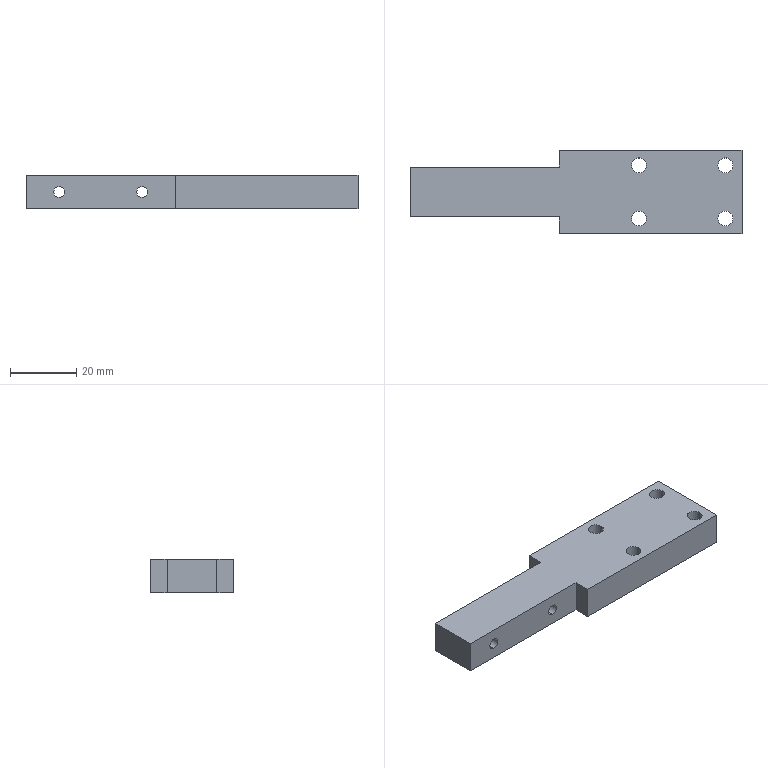Part | SolidWorks | features HoleWzd 2, Cut 1, Extrusion 1 | 1 solid | 34 faces | box 100 x 25 x 10 mm | volume 18975 mm3 | cylinder 20 | plane 14 | commonest cylinder face diameters 4.5 x8 8 x8 3.3 x4
STEP:
#1=CARTESIAN_POINT('',(-15.,-7.5,3.35));
#2=VERTEX_POINT('',#1);
#3=CARTESIAN_POINT('',(-15.,-7.5,6.65));
#4=VERTEX_POINT('',#3);
#5=CARTESIAN_POINT('',(-15.,-7.5,5.));
#6=DIRECTION('',(0.,1.,0.));
#7=DIRECTION('',(-1.,0.,0.));
#8=AXIS2_PLACEMENT_3D('',#5,#6,#7);
#9=CIRCLE('',#8,1.65);
#10=EDGE_CURVE('',#2,#4,#9,.T.);
#11=ORIENTED_EDGE('',*,*,#10,.F.);
#12=CARTESIAN_POINT('',(-15.,7.5,3.35));
#13=VERTEX_POINT('',#12);
#14=CARTESIAN_POINT('',(-15.,7.5,3.35));
#15=DIRECTION('',(0.,1.,0.));
#16=VECTOR('',#15,1000.);
#17=LINE('',#14,#16);
#18=EDGE_CURVE('',#2,#13,#17,.T.);
#19=ORIENTED_EDGE('',*,*,#18,.T.);
#20=CARTESIAN_POINT('',(-15.,7.5,6.65));
#21=VERTEX_POINT('',#20);
#22=CARTESIAN_POINT('',(-15.,7.5,5.));
#23=DIRECTION('',(0.,1.,0.));
#24=DIRECTION('',(0.,0.,1.));
#25=AXIS2_PLACEMENT_3D('',#22,#23,#24);
#26=CIRCLE('',#25,1.65);
#27=EDGE_CURVE('',#13,#21,#26,.T.);
#28=ORIENTED_EDGE('',*,*,#27,.T.);
#29=CARTESIAN_POINT('',(-15.,7.5,6.65));
#30=DIRECTION('',(0.,1.,0.));
#31=VECTOR('',#30,1000.);
#32=LINE('',#29,#31);
#33=EDGE_CURVE('',#4,#21,#32,.T.);
#34=ORIENTED_EDGE('',*,*,#33,.F.);
#35=EDGE_LOOP('',(#11,#19,#28,#34));
#36=FACE_OUTER_BOUND('',#35,.T.);
#37=CARTESIAN_POINT('',(-15.,7.5,5.));
#38=DIRECTION('',(0.,1.,0.));
#39=DIRECTION('',(0.,0.,1.));
#40=AXIS2_PLACEMENT_3D('',#37,#38,#39);
#41=CYLINDRICAL_SURFACE('',#40,1.65);
#42=ADVANCED_FACE('',(#36),#41,.F.);
#43=CARTESIAN_POINT('',(-40.,-7.5,3.35));
#44=VERTEX_POINT('',#43);
#45=CARTESIAN_POINT('',(-40.,-7.5,6.65));
#46=VERTEX_POINT('',#45);
#47=CARTESIAN_POINT('',(-40.,-7.5,5.));
#48=DIRECTION('',(0.,1.,0.));
#49=DIRECTION('',(-1.,0.,0.));
#50=AXIS2_PLACEMENT_3D('',#47,#48,#49);
#51=CIRCLE('',#50,1.65);
#52=EDGE_CURVE('',#44,#46,#51,.T.);
#53=ORIENTED_EDGE('',*,*,#52,.F.);
#54=CARTESIAN_POINT('',(-40.,7.5,3.35));
#55=VERTEX_POINT('',#54);
#56=CARTESIAN_POINT('',(-40.,7.5,3.35));
#57=DIRECTION('',(0.,1.,0.));
#58=VECTOR('',#57,1000.);
#59=LINE('',#56,#58);
#60=EDGE_CURVE('',#44,#55,#59,.T.);
#61=ORIENTED_EDGE('',*,*,#60,.T.);
#62=CARTESIAN_POINT('',(-40.,7.5,6.65));
#63=VERTEX_POINT('',#62);
#64=CARTESIAN_POINT('',(-40.,7.5,5.));
#65=DIRECTION('',(0.,1.,0.));
#66=DIRECTION('',(0.,0.,1.));
#67=AXIS2_PLACEMENT_3D('',#64,#65,#66);
#68=CIRCLE('',#67,1.65);
#69=EDGE_CURVE('',#55,#63,#68,.T.);
#70=ORIENTED_EDGE('',*,*,#69,.T.);
#71=CARTESIAN_POINT('',(-40.,7.5,6.65));
#72=DIRECTION('',(0.,1.,0.));
#73=VECTOR('',#72,1000.);
#74=LINE('',#71,#73);
#75=EDGE_CURVE('',#46,#63,#74,.T.);
#76=ORIENTED_EDGE('',*,*,#75,.F.);
#77=EDGE_LOOP('',(#53,#61,#70,#76));
#78=FACE_OUTER_BOUND('',#77,.T.);
#79=CARTESIAN_POINT('',(-40.,7.5,5.));
#80=DIRECTION('',(0.,1.,0.));
#81=DIRECTION('',(0.,0.,1.));
#82=AXIS2_PLACEMENT_3D('',#79,#80,#81);
#83=CYLINDRICAL_SURFACE('',#82,1.65);
#84=ADVANCED_FACE('',(#78),#83,.F.);
#85=CARTESIAN_POINT('',(23.,-8.,4.6));
#86=VERTEX_POINT('',#85);
#87=CARTESIAN_POINT('',(15.,-8.,4.6));
#88=VERTEX_POINT('',#87);
#89=CARTESIAN_POINT('',(19.,-8.,4.6));
#90=DIRECTION('',(0.,0.,-1.));
#91=DIRECTION('',(-1.,0.,0.));
#92=AXIS2_PLACEMENT_3D('',#89,#90,#91);
#93=CIRCLE('',#92,4.);
#94=EDGE_CURVE('',#86,#88,#93,.T.);
#95=ORIENTED_EDGE('',*,*,#94,.F.);
#96=CARTESIAN_POINT('',(23.,-8.,0.));
#97=VERTEX_POINT('',#96);
#98=CARTESIAN_POINT('',(23.,-8.,0.));
#99=DIRECTION('',(0.,0.,-1.));
#100=VECTOR('',#99,1000.);
#101=LINE('',#98,#100);
#102=EDGE_CURVE('',#86,#97,#101,.T.);
#103=ORIENTED_EDGE('',*,*,#102,.T.);
#104=CARTESIAN_POINT('',(15.,-8.,0.));
#105=VERTEX_POINT('',#104);
#106=CARTESIAN_POINT('',(19.,-8.,0.));
#107=DIRECTION('',(0.,0.,-1.));
#108=DIRECTION('',(-1.,0.,0.));
#109=AXIS2_PLACEMENT_3D('',#106,#107,#108);
#110=CIRCLE('',#109,4.);
#111=EDGE_CURVE('',#97,#105,#110,.T.);
#112=ORIENTED_EDGE('',*,*,#111,.T.);
#113=CARTESIAN_POINT('',(15.,-8.,0.));
#114=DIRECTION('',(0.,0.,-1.));
#115=VECTOR('',#114,1000.);
#116=LINE('',#113,#115);
#117=EDGE_CURVE('',#88,#105,#116,.T.);
#118=ORIENTED_EDGE('',*,*,#117,.F.);
#119=EDGE_LOOP('',(#95,#103,#112,#118));
#120=FACE_OUTER_BOUND('',#119,.T.);
#121=CARTESIAN_POINT('',(19.,-8.,0.));
#122=DIRECTION('',(0.,0.,-1.));
#123=DIRECTION('',(-1.,0.,0.));
#124=AXIS2_PLACEMENT_3D('',#121,#122,#123);
#125=CYLINDRICAL_SURFACE('',#124,4.);
#126=ADVANCED_FACE('',(#120),#125,.F.);
#127=CARTESIAN_POINT('',(21.25,-8.,10.));
#128=VERTEX_POINT('',#127);
#129=CARTESIAN_POINT('',(16.75,-8.,10.));
#130=VERTEX_POINT('',#129);
#131=CARTESIAN_POINT('',(19.,-8.,10.));
#132=DIRECTION('',(0.,0.,-1.));
#133=DIRECTION('',(-1.,0.,0.));
#134=AXIS2_PLACEMENT_3D('',#131,#132,#133);
#135=CIRCLE('',#134,2.25);
#136=EDGE_CURVE('',#128,#130,#135,.T.);
#137=ORIENTED_EDGE('',*,*,#136,.F.);
#138=CARTESIAN_POINT('',(21.25,-8.,4.6));
#139=VERTEX_POINT('',#138);
#140=CARTESIAN_POINT('',(21.25,-8.,0.));
#141=DIRECTION('',(0.,0.,-1.));
#142=VECTOR('',#141,1000.);
#143=LINE('',#140,#142);
#144=EDGE_CURVE('',#128,#139,#143,.T.);
#145=ORIENTED_EDGE('',*,*,#144,.T.);
#146=CARTESIAN_POINT('',(16.75,-8.,4.6));
#147=VERTEX_POINT('',#146);
#148=CARTESIAN_POINT('',(19.,-8.,4.6));
#149=DIRECTION('',(0.,0.,-1.));
#150=DIRECTION('',(-1.,0.,0.));
#151=AXIS2_PLACEMENT_3D('',#148,#149,#150);
#152=CIRCLE('',#151,2.25);
#153=EDGE_CURVE('',#139,#147,#152,.T.);
#154=ORIENTED_EDGE('',*,*,#153,.T.);
#155=CARTESIAN_POINT('',(16.75,-8.,0.));
#156=DIRECTION('',(0.,0.,-1.));
#157=VECTOR('',#156,1000.);
#158=LINE('',#155,#157);
#159=EDGE_CURVE('',#130,#147,#158,.T.);
#160=ORIENTED_EDGE('',*,*,#159,.F.);
#161=EDGE_LOOP('',(#137,#145,#154,#160));
#162=FACE_OUTER_BOUND('',#161,.T.);
#163=CARTESIAN_POINT('',(19.,-8.,0.));
#164=DIRECTION('',(0.,0.,-1.));
#165=DIRECTION('',(-1.,0.,0.));
#166=AXIS2_PLACEMENT_3D('',#163,#164,#165);
#167=CYLINDRICAL_SURFACE('',#166,2.25);
#168=ADVANCED_FACE('',(#162),#167,.F.);
#169=CARTESIAN_POINT('',(23.,8.,4.6));
#170=VERTEX_POINT('',#169);
#171=CARTESIAN_POINT('',(15.,8.,4.6));
#172=VERTEX_POINT('',#171);
#173=CARTESIAN_POINT('',(19.,8.,4.6));
#174=DIRECTION('',(0.,0.,-1.));
#175=DIRECTION('',(-1.,0.,0.));
#176=AXIS2_PLACEMENT_3D('',#173,#174,#175);
#177=CIRCLE('',#176,4.);
#178=EDGE_CURVE('',#170,#172,#177,.T.);
#179=ORIENTED_EDGE('',*,*,#178,.F.);
#180=CARTESIAN_POINT('',(23.,8.,0.));
#181=VERTEX_POINT('',#180);
#182=CARTESIAN_POINT('',(23.,8.,0.));
#183=DIRECTION('',(0.,0.,-1.));
#184=VECTOR('',#183,1000.);
#185=LINE('',#182,#184);
#186=EDGE_CURVE('',#170,#181,#185,.T.);
#187=ORIENTED_EDGE('',*,*,#186,.T.);
#188=CARTESIAN_POINT('',(15.,8.,0.));
#189=VERTEX_POINT('',#188);
#190=CARTESIAN_POINT('',(19.,8.,0.));
#191=DIRECTION('',(0.,0.,-1.));
#192=DIRECTION('',(-1.,0.,0.));
#193=AXIS2_PLACEMENT_3D('',#190,#191,#192);
#194=CIRCLE('',#193,4.);
#195=EDGE_CURVE('',#181,#189,#194,.T.);
#196=ORIENTED_EDGE('',*,*,#195,.T.);
#197=CARTESIAN_POINT('',(15.,8.,0.));
#198=DIRECTION('',(0.,0.,-1.));
#199=VECTOR('',#198,1000.);
#200=LINE('',#197,#199);
#201=EDGE_CURVE('',#172,#189,#200,.T.);
#202=ORIENTED_EDGE('',*,*,#201,.F.);
#203=EDGE_LOOP('',(#179,#187,#196,#202));
#204=FACE_OUTER_BOUND('',#203,.T.);
#205=CARTESIAN_POINT('',(19.,8.,0.));
#206=DIRECTION('',(0.,0.,-1.));
#207=DIRECTION('',(-1.,0.,0.));
#208=AXIS2_PLACEMENT_3D('',#205,#206,#207);
#209=CYLINDRICAL_SURFACE('',#208,4.);
#210=ADVANCED_FACE('',(#204),#209,.F.);
#211=CARTESIAN_POINT('',(21.25,8.,10.));
#212=VERTEX_POINT('',#211);
#213=CARTESIAN_POINT('',(16.75,8.,10.));
#214=VERTEX_POINT('',#213);
#215=CARTESIAN_POINT('',(19.,8.,10.));
#216=DIRECTION('',(0.,0.,-1.));
#217=DIRECTION('',(-1.,0.,0.));
#218=AXIS2_PLACEMENT_3D('',#215,#216,#217);
#219=CIRCLE('',#218,2.25);
#220=EDGE_CURVE('',#212,#214,#219,.T.);
#221=ORIENTED_EDGE('',*,*,#220,.F.);
#222=CARTESIAN_POINT('',(21.25,8.,4.6));
#223=VERTEX_POINT('',#222);
#224=CARTESIAN_POINT('',(21.25,8.,0.));
#225=DIRECTION('',(0.,0.,-1.));
#226=VECTOR('',#225,1000.);
#227=LINE('',#224,#226);
#228=EDGE_CURVE('',#212,#223,#227,.T.);
#229=ORIENTED_EDGE('',*,*,#228,.T.);
#230=CARTESIAN_POINT('',(16.75,8.,4.6));
#231=VERTEX_POINT('',#230);
#232=CARTESIAN_POINT('',(19.,8.,4.6));
#233=DIRECTION('',(0.,0.,-1.));
#234=DIRECTION('',(-1.,0.,0.));
#235=AXIS2_PLACEMENT_3D('',#232,#233,#234);
#236=CIRCLE('',#235,2.25);
#237=EDGE_CURVE('',#223,#231,#236,.T.);
#238=ORIENTED_EDGE('',*,*,#237,.T.);
#239=CARTESIAN_POINT('',(16.75,8.,0.));
#240=DIRECTION('',(0.,0.,-1.));
#241=VECTOR('',#240,1000.);
#242=LINE('',#239,#241);
#243=EDGE_CURVE('',#214,#231,#242,.T.);
#244=ORIENTED_EDGE('',*,*,#243,.F.);
#245=EDGE_LOOP('',(#221,#229,#238,#244));
#246=FACE_OUTER_BOUND('',#245,.T.);
#247=CARTESIAN_POINT('',(19.,8.,0.));
#248=DIRECTION('',(0.,0.,-1.));
#249=DIRECTION('',(-1.,0.,0.));
#250=AXIS2_PLACEMENT_3D('',#247,#248,#249);
#251=CYLINDRICAL_SURFACE('',#250,2.25);
#252=ADVANCED_FACE('',(#246),#251,.F.);
#253=CARTESIAN_POINT('',(49.,8.,4.6));
#254=VERTEX_POINT('',#253);
#255=CARTESIAN_POINT('',(41.,8.,4.6));
#256=VERTEX_POINT('',#255);
#257=CARTESIAN_POINT('',(45.,8.,4.6));
#258=DIRECTION('',(0.,0.,-1.));
#259=DIRECTION('',(-1.,0.,0.));
#260=AXIS2_PLACEMENT_3D('',#257,#258,#259);
#261=CIRCLE('',#260,4.);
#262=EDGE_CURVE('',#254,#256,#261,.T.);
#263=ORIENTED_EDGE('',*,*,#262,.F.);
#264=CARTESIAN_POINT('',(49.,8.,0.));
#265=VERTEX_POINT('',#264);
#266=CARTESIAN_POINT('',(49.,8.,0.));
#267=DIRECTION('',(0.,0.,-1.));
#268=VECTOR('',#267,1000.);
#269=LINE('',#266,#268);
#270=EDGE_CURVE('',#254,#265,#269,.T.);
#271=ORIENTED_EDGE('',*,*,#270,.T.);
#272=CARTESIAN_POINT('',(41.,8.,0.));
#273=VERTEX_POINT('',#272);
#274=CARTESIAN_POINT('',(45.,8.,0.));
#275=DIRECTION('',(0.,0.,-1.));
#276=DIRECTION('',(-1.,0.,0.));
#277=AXIS2_PLACEMENT_3D('',#274,#275,#276);
#278=CIRCLE('',#277,4.);
#279=EDGE_CURVE('',#265,#273,#278,.T.);
#280=ORIENTED_EDGE('',*,*,#279,.T.);
#281=CARTESIAN_POINT('',(41.,8.,0.));
#282=DIRECTION('',(0.,0.,-1.));
#283=VECTOR('',#282,1000.);
#284=LINE('',#281,#283);
#285=EDGE_CURVE('',#256,#273,#284,.T.);
#286=ORIENTED_EDGE('',*,*,#285,.F.);
#287=EDGE_LOOP('',(#263,#271,#280,#286));
#288=FACE_OUTER_BOUND('',#287,.T.);
#289=CARTESIAN_POINT('',(45.,8.,0.));
#290=DIRECTION('',(0.,0.,-1.));
#291=DIRECTION('',(-1.,0.,0.));
#292=AXIS2_PLACEMENT_3D('',#289,#290,#291);
#293=CYLINDRICAL_SURFACE('',#292,4.);
#294=ADVANCED_FACE('',(#288),#293,.F.);
#295=CARTESIAN_POINT('',(47.25,8.,10.));
#296=VERTEX_POINT('',#295);
#297=CARTESIAN_POINT('',(42.75,8.,10.));
#298=VERTEX_POINT('',#297);
#299=CARTESIAN_POINT('',(45.,8.,10.));
#300=DIRECTION('',(0.,0.,-1.));
#301=DIRECTION('',(-1.,0.,0.));
#302=AXIS2_PLACEMENT_3D('',#299,#300,#301);
#303=CIRCLE('',#302,2.25);
#304=EDGE_CURVE('',#296,#298,#303,.T.);
#305=ORIENTED_EDGE('',*,*,#304,.F.);
#306=CARTESIAN_POINT('',(47.25,8.,4.6));
#307=VERTEX_POINT('',#306);
#308=CARTESIAN_POINT('',(47.25,8.,0.));
#309=DIRECTION('',(0.,0.,-1.));
#310=VECTOR('',#309,1000.);
#311=LINE('',#308,#310);
#312=EDGE_CURVE('',#296,#307,#311,.T.);
#313=ORIENTED_EDGE('',*,*,#312,.T.);
#314=CARTESIAN_POINT('',(42.75,8.,4.6));
#315=VERTEX_POINT('',#314);
#316=CARTESIAN_POINT('',(45.,8.,4.6));
#317=DIRECTION('',(0.,0.,-1.));
#318=DIRECTION('',(-1.,0.,0.));
#319=AXIS2_PLACEMENT_3D('',#316,#317,#318);
#320=CIRCLE('',#319,2.25);
#321=EDGE_CURVE('',#307,#315,#320,.T.);
#322=ORIENTED_EDGE('',*,*,#321,.T.);
#323=CARTESIAN_POINT('',(42.75,8.,0.));
#324=DIRECTION('',(0.,0.,-1.));
#325=VECTOR('',#324,1000.);
#326=LINE('',#323,#325);
#327=EDGE_CURVE('',#298,#315,#326,.T.);
#328=ORIENTED_EDGE('',*,*,#327,.F.);
#329=EDGE_LOOP('',(#305,#313,#322,#328));
#330=FACE_OUTER_BOUND('',#329,.T.);
#331=CARTESIAN_POINT('',(45.,8.,0.));
#332=DIRECTION('',(0.,0.,-1.));
#333=DIRECTION('',(-1.,0.,0.));
#334=AXIS2_PLACEMENT_3D('',#331,#332,#333);
#335=CYLINDRICAL_SURFACE('',#334,2.25);
#336=ADVANCED_FACE('',(#330),#335,.F.);
#337=CARTESIAN_POINT('',(49.,-8.,4.6));
#338=VERTEX_POINT('',#337);
#339=CARTESIAN_POINT('',(41.,-8.,4.6));
#340=VERTEX_POINT('',#339);
#341=CARTESIAN_POINT('',(45.,-8.,4.6));
#342=DIRECTION('',(0.,0.,-1.));
#343=DIRECTION('',(-1.,0.,0.));
#344=AXIS2_PLACEMENT_3D('',#341,#342,#343);
#345=CIRCLE('',#344,4.);
#346=EDGE_CURVE('',#338,#340,#345,.T.);
#347=ORIENTED_EDGE('',*,*,#346,.F.);
#348=CARTESIAN_POINT('',(49.,-8.,0.));
#349=VERTEX_POINT('',#348);
#350=CARTESIAN_POINT('',(49.,-8.,0.));
#351=DIRECTION('',(0.,0.,-1.));
#352=VECTOR('',#351,1000.);
#353=LINE('',#350,#352);
#354=EDGE_CURVE('',#338,#349,#353,.T.);
#355=ORIENTED_EDGE('',*,*,#354,.T.);
#356=CARTESIAN_POINT('',(41.,-8.,0.));
#357=VERTEX_POINT('',#356);
#358=CARTESIAN_POINT('',(45.,-8.,0.));
#359=DIRECTION('',(0.,0.,-1.));
#360=DIRECTION('',(-1.,0.,0.));
#361=AXIS2_PLACEMENT_3D('',#358,#359,#360);
#362=CIRCLE('',#361,4.);
#363=EDGE_CURVE('',#349,#357,#362,.T.);
#364=ORIENTED_EDGE('',*,*,#363,.T.);
#365=CARTESIAN_POINT('',(41.,-8.,0.));
#366=DIRECTION('',(0.,0.,-1.));
#367=VECTOR('',#366,1000.);
#368=LINE('',#365,#367);
#369=EDGE_CURVE('',#340,#357,#368,.T.);
#370=ORIENTED_EDGE('',*,*,#369,.F.);
#371=EDGE_LOOP('',(#347,#355,#364,#370));
#372=FACE_OUTER_BOUND('',#371,.T.);
#373=CARTESIAN_POINT('',(45.,-8.,0.));
#374=DIRECTION('',(0.,0.,-1.));
#375=DIRECTION('',(-1.,0.,0.));
#376=AXIS2_PLACEMENT_3D('',#373,#374,#375);
#377=CYLINDRICAL_SURFACE('',#376,4.);
#378=ADVANCED_FACE('',(#372),#377,.F.);
#379=CARTESIAN_POINT('',(47.25,-8.,10.));
#380=VERTEX_POINT('',#379);
#381=CARTESIAN_POINT('',(42.75,-8.,10.));
#382=VERTEX_POINT('',#381);
#383=CARTESIAN_POINT('',(45.,-8.,10.));
#384=DIRECTION('',(0.,0.,-1.));
#385=DIRECTION('',(-1.,0.,0.));
#386=AXIS2_PLACEMENT_3D('',#383,#384,#385);
#387=CIRCLE('',#386,2.25);
#388=EDGE_CURVE('',#380,#382,#387,.T.);
#389=ORIENTED_EDGE('',*,*,#388,.F.);
#390=CARTESIAN_POINT('',(47.25,-8.,4.6));
#391=VERTEX_POINT('',#390);
#392=CARTESIAN_POINT('',(47.25,-8.,0.));
#393=DIRECTION('',(0.,0.,-1.));
#394=VECTOR('',#393,1000.);
#395=LINE('',#392,#394);
#396=EDGE_CURVE('',#380,#391,#395,.T.);
#397=ORIENTED_EDGE('',*,*,#396,.T.);
#398=CARTESIAN_POINT('',(42.75,-8.,4.6));
#399=VERTEX_POINT('',#398);
#400=CARTESIAN_POINT('',(45.,-8.,4.6));
#401=DIRECTION('',(0.,0.,-1.));
#402=DIRECTION('',(-1.,0.,0.));
#403=AXIS2_PLACEMENT_3D('',#400,#401,#402);
#404=CIRCLE('',#403,2.25);
#405=EDGE_CURVE('',#391,#399,#404,.T.);
#406=ORIENTED_EDGE('',*,*,#405,.T.);
#407=CARTESIAN_POINT('',(42.75,-8.,0.));
#408=DIRECTION('',(0.,0.,-1.));
#409=VECTOR('',#408,1000.);
#410=LINE('',#407,#409);
#411=EDGE_CURVE('',#382,#399,#410,.T.);
#412=ORIENTED_EDGE('',*,*,#411,.F.);
#413=EDGE_LOOP('',(#389,#397,#406,#412));
#414=FACE_OUTER_BOUND('',#413,.T.);
#415=CARTESIAN_POINT('',(45.,-8.,0.));
#416=DIRECTION('',(0.,0.,-1.));
#417=DIRECTION('',(-1.,0.,0.));
#418=AXIS2_PLACEMENT_3D('',#415,#416,#417);
#419=CYLINDRICAL_SURFACE('',#418,2.25);
#420=ADVANCED_FACE('',(#414),#419,.F.);
#421=CARTESIAN_POINT('',(50.,-12.5,0.));
#422=VERTEX_POINT('',#421);
#423=CARTESIAN_POINT('',(50.,12.5,0.));
#424=VERTEX_POINT('',#423);
#425=CARTESIAN_POINT('',(50.,12.5,0.));
#426=DIRECTION('',(0.,1.,0.));
#427=VECTOR('',#426,1000.);
#428=LINE('',#425,#427);
#429=EDGE_CURVE('',#422,#424,#428,.T.);
#430=ORIENTED_EDGE('',*,*,#429,.T.);
#431=CARTESIAN_POINT('',(50.,12.5,10.));
#432=VERTEX_POINT('',#431);
#433=CARTESIAN_POINT('',(50.,12.5,10.));
#434=DIRECTION('',(0.,0.,-1.));
#435=VECTOR('',#434,1000.);
#436=LINE('',#433,#435);
#437=EDGE_CURVE('',#432,#424,#436,.T.);
#438=ORIENTED_EDGE('',*,*,#437,.F.);
#439=CARTESIAN_POINT('',(50.,-12.5,10.));
#440=VERTEX_POINT('',#439);
#441=CARTESIAN_POINT('',(50.,12.5,10.));
#442=DIRECTION('',(0.,1.,0.));
#443=VECTOR('',#442,1000.);
#444=LINE('',#441,#443);
#445=EDGE_CURVE('',#440,#432,#444,.T.);
#446=ORIENTED_EDGE('',*,*,#445,.F.);
#447=CARTESIAN_POINT('',(50.,-12.5,10.));
#448=DIRECTION('',(0.,0.,-1.));
#449=VECTOR('',#448,1000.);
#450=LINE('',#447,#449);
#451=EDGE_CURVE('',#440,#422,#450,.T.);
#452=ORIENTED_EDGE('',*,*,#451,.T.);
#453=EDGE_LOOP('',(#430,#438,#446,#452));
#454=FACE_OUTER_BOUND('',#453,.T.);
#455=CARTESIAN_POINT('',(50.,12.5,10.));
#456=DIRECTION('',(-1.,0.,0.));
#457=DIRECTION('',(0.,0.,1.));
#458=AXIS2_PLACEMENT_3D('',#455,#456,#457);
#459=PLANE('',#458);
#460=ADVANCED_FACE('',(#454),#459,.F.);
#461=CARTESIAN_POINT('',(-5.,12.5,0.));
#462=VERTEX_POINT('',#461);
#463=CARTESIAN_POINT('',(-50.,12.5,0.));
#464=DIRECTION('',(-1.,0.,0.));
#465=VECTOR('',#464,1000.);
#466=LINE('',#463,#465);
#467=EDGE_CURVE('',#424,#462,#466,.T.);
#468=ORIENTED_EDGE('',*,*,#467,.T.);
#469=CARTESIAN_POINT('',(-5.,12.5,10.));
#470=VERTEX_POINT('',#469);
#471=CARTESIAN_POINT('',(-5.,12.5,10.));
#472=DIRECTION('',(0.,0.,-1.));
#473=VECTOR('',#472,1000.);
#474=LINE('',#471,#473);
#475=EDGE_CURVE('',#470,#462,#474,.T.);
#476=ORIENTED_EDGE('',*,*,#475,.F.);
#477=CARTESIAN_POINT('',(-50.,12.5,10.));
#478=DIRECTION('',(-1.,0.,0.));
#479=VECTOR('',#478,1000.);
#480=LINE('',#477,#479);
#481=EDGE_CURVE('',#432,#470,#480,.T.);
#482=ORIENTED_EDGE('',*,*,#481,.F.);
#483=ORIENTED_EDGE('',*,*,#437,.T.);
#484=EDGE_LOOP('',(#468,#476,#482,#483));
#485=FACE_OUTER_BOUND('',#484,.T.);
#486=CARTESIAN_POINT('',(-50.,12.5,10.));
#487=DIRECTION('',(0.,-1.,0.));
#488=DIRECTION('',(0.,0.,-1.));
#489=AXIS2_PLACEMENT_3D('',#486,#487,#488);
#490=PLANE('',#489);
#491=ADVANCED_FACE('',(#485),#490,.F.);
#492=CARTESIAN_POINT('',(-50.,7.5,10.));
#493=VERTEX_POINT('',#492);
#494=CARTESIAN_POINT('',(-50.,-7.5,10.));
#495=VERTEX_POINT('',#494);
#496=CARTESIAN_POINT('',(-50.,12.5,10.));
#497=DIRECTION('',(0.,-1.,0.));
#498=VECTOR('',#497,1000.);
#499=LINE('',#496,#498);
#500=EDGE_CURVE('',#493,#495,#499,.T.);
#501=ORIENTED_EDGE('',*,*,#500,.F.);
#502=CARTESIAN_POINT('',(-50.,7.5,0.));
#503=VERTEX_POINT('',#502);
#504=CARTESIAN_POINT('',(-50.,7.5,10.));
#505=DIRECTION('',(0.,0.,-1.));
#506=VECTOR('',#505,1000.);
#507=LINE('',#504,#506);
#508=EDGE_CURVE('',#493,#503,#507,.T.);
#509=ORIENTED_EDGE('',*,*,#508,.T.);
#510=CARTESIAN_POINT('',(-50.,-7.5,0.));
#511=VERTEX_POINT('',#510);
#512=CARTESIAN_POINT('',(-50.,12.5,0.));
#513=DIRECTION('',(0.,-1.,0.));
#514=VECTOR('',#513,1000.);
#515=LINE('',#512,#514);
#516=EDGE_CURVE('',#503,#511,#515,.T.);
#517=ORIENTED_EDGE('',*,*,#516,.T.);
#518=CARTESIAN_POINT('',(-50.,-7.5,10.));
#519=DIRECTION('',(0.,0.,-1.));
#520=VECTOR('',#519,1000.);
#521=LINE('',#518,#520);
#522=EDGE_CURVE('',#495,#511,#521,.T.);
#523=ORIENTED_EDGE('',*,*,#522,.F.);
#524=EDGE_LOOP('',(#501,#509,#517,#523));
#525=FACE_OUTER_BOUND('',#524,.T.);
#526=CARTESIAN_POINT('',(-50.,12.5,10.));
#527=DIRECTION('',(1.,0.,0.));
#528=DIRECTION('',(0.,0.,-1.));
#529=AXIS2_PLACEMENT_3D('',#526,#527,#528);
#530=PLANE('',#529);
#531=ADVANCED_FACE('',(#525),#530,.F.);
#532=CARTESIAN_POINT('',(-5.,-12.5,10.));
#533=VERTEX_POINT('',#532);
#534=CARTESIAN_POINT('',(-50.,-12.5,10.));
#535=DIRECTION('',(1.,0.,0.));
#536=VECTOR('',#535,1000.);
#537=LINE('',#534,#536);
#538=EDGE_CURVE('',#533,#440,#537,.T.);
#539=ORIENTED_EDGE('',*,*,#538,.F.);
#540=CARTESIAN_POINT('',(-5.,-12.5,0.));
#541=VERTEX_POINT('',#540);
#542=CARTESIAN_POINT('',(-5.,-12.5,10.));
#543=DIRECTION('',(0.,0.,-1.));
#544=VECTOR('',#543,1000.);
#545=LINE('',#542,#544);
#546=EDGE_CURVE('',#533,#541,#545,.T.);
#547=ORIENTED_EDGE('',*,*,#546,.T.);
#548=CARTESIAN_POINT('',(-50.,-12.5,0.));
#549=DIRECTION('',(1.,0.,0.));
#550=VECTOR('',#549,1000.);
#551=LINE('',#548,#550);
#552=EDGE_CURVE('',#541,#422,#551,.T.);
#553=ORIENTED_EDGE('',*,*,#552,.T.);
#554=ORIENTED_EDGE('',*,*,#451,.F.);
#555=EDGE_LOOP('',(#539,#547,#553,#554));
#556=FACE_OUTER_BOUND('',#555,.T.);
#557=CARTESIAN_POINT('',(-50.,-12.5,10.));
#558=DIRECTION('',(0.,1.,0.));
#559=DIRECTION('',(0.,0.,1.));
#560=AXIS2_PLACEMENT_3D('',#557,#558,#559);
#561=PLANE('',#560);
#562=ADVANCED_FACE('',(#556),#561,.F.);
#563=CARTESIAN_POINT('',(19.,-8.,10.));
#564=DIRECTION('',(0.,0.,-1.));
#565=DIRECTION('',(-1.,0.,0.));
#566=AXIS2_PLACEMENT_3D('',#563,#564,#565);
#567=CIRCLE('',#566,2.25);
#568=EDGE_CURVE('',#130,#128,#567,.T.);
#569=ORIENTED_EDGE('',*,*,#568,.T.);
#570=ORIENTED_EDGE('',*,*,#136,.T.);
#571=EDGE_LOOP('',(#569,#570));
#572=FACE_BOUND('',#571,.T.);
#573=CARTESIAN_POINT('',(19.,8.,10.));
#574=DIRECTION('',(0.,0.,-1.));
#575=DIRECTION('',(-1.,0.,0.));
#576=AXIS2_PLACEMENT_3D('',#573,#574,#575);
#577=CIRCLE('',#576,2.25);
#578=EDGE_CURVE('',#214,#212,#577,.T.);
#579=ORIENTED_EDGE('',*,*,#578,.T.);
#580=ORIENTED_EDGE('',*,*,#220,.T.);
#581=EDGE_LOOP('',(#579,#580));
#582=FACE_BOUND('',#581,.T.);
#583=CARTESIAN_POINT('',(45.,8.,10.));
#584=DIRECTION('',(0.,0.,-1.));
#585=DIRECTION('',(-1.,0.,0.));
#586=AXIS2_PLACEMENT_3D('',#583,#584,#585);
#587=CIRCLE('',#586,2.25);
#588=EDGE_CURVE('',#298,#296,#587,.T.);
#589=ORIENTED_EDGE('',*,*,#588,.T.);
#590=ORIENTED_EDGE('',*,*,#304,.T.);
#591=EDGE_LOOP('',(#589,#590));
#592=FACE_BOUND('',#591,.T.);
#593=CARTESIAN_POINT('',(45.,-8.,10.));
#594=DIRECTION('',(0.,0.,-1.));
#595=DIRECTION('',(-1.,0.,0.));
#596=AXIS2_PLACEMENT_3D('',#593,#594,#595);
#597=CIRCLE('',#596,2.25);
#598=EDGE_CURVE('',#382,#380,#597,.T.);
#599=ORIENTED_EDGE('',*,*,#598,.T.);
#600=ORIENTED_EDGE('',*,*,#388,.T.);
#601=EDGE_LOOP('',(#599,#600));
#602=FACE_BOUND('',#601,.T.);
#603=CARTESIAN_POINT('',(-5.,7.5,10.));
#604=VERTEX_POINT('',#603);
#605=CARTESIAN_POINT('',(-50.,7.5,10.));
#606=DIRECTION('',(-1.,0.,0.));
#607=VECTOR('',#606,1000.);
#608=LINE('',#605,#607);
#609=EDGE_CURVE('',#604,#493,#608,.T.);
#610=ORIENTED_EDGE('',*,*,#609,.T.);
#611=ORIENTED_EDGE('',*,*,#500,.T.);
#612=CARTESIAN_POINT('',(-5.,-7.5,10.));
#613=VERTEX_POINT('',#612);
#614=CARTESIAN_POINT('',(-50.,-7.5,10.));
#615=DIRECTION('',(1.,0.,0.));
#616=VECTOR('',#615,1000.);
#617=LINE('',#614,#616);
#618=EDGE_CURVE('',#495,#613,#617,.T.);
#619=ORIENTED_EDGE('',*,*,#618,.T.);
#620=CARTESIAN_POINT('',(-5.,-12.5,10.));
#621=DIRECTION('',(0.,-1.,0.));
#622=VECTOR('',#621,1000.);
#623=LINE('',#620,#622);
#624=EDGE_CURVE('',#613,#533,#623,.T.);
#625=ORIENTED_EDGE('',*,*,#624,.T.);
#626=ORIENTED_EDGE('',*,*,#538,.T.);
#627=ORIENTED_EDGE('',*,*,#445,.T.);
#628=ORIENTED_EDGE('',*,*,#481,.T.);
#629=CARTESIAN_POINT('',(-5.,12.5,10.));
#630=DIRECTION('',(0.,-1.,0.));
#631=VECTOR('',#630,1000.);
#632=LINE('',#629,#631);
#633=EDGE_CURVE('',#470,#604,#632,.T.);
#634=ORIENTED_EDGE('',*,*,#633,.T.);
#635=EDGE_LOOP('',(#610,#611,#619,#625,#626,#627,#628,#634));
#636=FACE_OUTER_BOUND('',#635,.T.);
#637=CARTESIAN_POINT('',(0.,0.,10.));
#638=DIRECTION('',(0.,0.,1.));
#639=DIRECTION('',(1.,0.,0.));
#640=AXIS2_PLACEMENT_3D('',#637,#638,#639);
#641=PLANE('',#640);
#642=ADVANCED_FACE('',(#572,#582,#592,#602,#636),#641,.T.);
#643=CARTESIAN_POINT('',(19.,-8.,0.));
#644=DIRECTION('',(0.,0.,-1.));
#645=DIRECTION('',(-1.,0.,0.));
#646=AXIS2_PLACEMENT_3D('',#643,#644,#645);
#647=CIRCLE('',#646,4.);
#648=EDGE_CURVE('',#105,#97,#647,.T.);
#649=ORIENTED_EDGE('',*,*,#648,.F.);
#650=ORIENTED_EDGE('',*,*,#111,.F.);
#651=EDGE_LOOP('',(#649,#650));
#652=FACE_BOUND('',#651,.T.);
#653=CARTESIAN_POINT('',(19.,8.,0.));
#654=DIRECTION('',(0.,0.,-1.));
#655=DIRECTION('',(-1.,0.,0.));
#656=AXIS2_PLACEMENT_3D('',#653,#654,#655);
#657=CIRCLE('',#656,4.);
#658=EDGE_CURVE('',#189,#181,#657,.T.);
#659=ORIENTED_EDGE('',*,*,#658,.F.);
#660=ORIENTED_EDGE('',*,*,#195,.F.);
#661=EDGE_LOOP('',(#659,#660));
#662=FACE_BOUND('',#661,.T.);
#663=CARTESIAN_POINT('',(45.,8.,0.));
#664=DIRECTION('',(0.,0.,-1.));
#665=DIRECTION('',(-1.,0.,0.));
#666=AXIS2_PLACEMENT_3D('',#663,#664,#665);
#667=CIRCLE('',#666,4.);
#668=EDGE_CURVE('',#273,#265,#667,.T.);
#669=ORIENTED_EDGE('',*,*,#668,.F.);
#670=ORIENTED_EDGE('',*,*,#279,.F.);
#671=EDGE_LOOP('',(#669,#670));
#672=FACE_BOUND('',#671,.T.);
#673=CARTESIAN_POINT('',(45.,-8.,0.));
#674=DIRECTION('',(0.,0.,-1.));
#675=DIRECTION('',(-1.,0.,0.));
#676=AXIS2_PLACEMENT_3D('',#673,#674,#675);
#677=CIRCLE('',#676,4.);
#678=EDGE_CURVE('',#357,#349,#677,.T.);
#679=ORIENTED_EDGE('',*,*,#678,.F.);
#680=ORIENTED_EDGE('',*,*,#363,.F.);
#681=EDGE_LOOP('',(#679,#680));
#682=FACE_BOUND('',#681,.T.);
#683=ORIENTED_EDGE('',*,*,#516,.F.);
#684=CARTESIAN_POINT('',(-5.,7.5,0.));
#685=VERTEX_POINT('',#684);
#686=CARTESIAN_POINT('',(0.,7.5,0.));
#687=DIRECTION('',(1.,0.,0.));
#688=VECTOR('',#687,1000.);
#689=LINE('',#686,#688);
#690=EDGE_CURVE('',#503,#685,#689,.T.);
#691=ORIENTED_EDGE('',*,*,#690,.T.);
#692=CARTESIAN_POINT('',(-5.,0.,0.));
#693=DIRECTION('',(0.,1.,0.));
#694=VECTOR('',#693,1000.);
#695=LINE('',#692,#694);
#696=EDGE_CURVE('',#685,#462,#695,.T.);
#697=ORIENTED_EDGE('',*,*,#696,.T.);
#698=ORIENTED_EDGE('',*,*,#467,.F.);
#699=ORIENTED_EDGE('',*,*,#429,.F.);
#700=ORIENTED_EDGE('',*,*,#552,.F.);
#701=CARTESIAN_POINT('',(-5.,-7.5,0.));
#702=VERTEX_POINT('',#701);
#703=CARTESIAN_POINT('',(-5.,0.,0.));
#704=DIRECTION('',(0.,1.,0.));
#705=VECTOR('',#704,1000.);
#706=LINE('',#703,#705);
#707=EDGE_CURVE('',#541,#702,#706,.T.);
#708=ORIENTED_EDGE('',*,*,#707,.T.);
#709=CARTESIAN_POINT('',(0.,-7.5,0.));
#710=DIRECTION('',(-1.,0.,0.));
#711=VECTOR('',#710,1000.);
#712=LINE('',#709,#711);
#713=EDGE_CURVE('',#702,#511,#712,.T.);
#714=ORIENTED_EDGE('',*,*,#713,.T.);
#715=EDGE_LOOP('',(#683,#691,#697,#698,#699,#700,#708,#714));
#716=FACE_OUTER_BOUND('',#715,.T.);
#717=CARTESIAN_POINT('',(0.,0.,0.));
#718=DIRECTION('',(0.,0.,1.));
#719=DIRECTION('',(1.,0.,0.));
#720=AXIS2_PLACEMENT_3D('',#717,#718,#719);
#721=PLANE('',#720);
#722=ADVANCED_FACE('',(#652,#662,#672,#682,#716),#721,.F.);
#723=ORIENTED_EDGE('',*,*,#546,.F.);
#724=ORIENTED_EDGE('',*,*,#624,.F.);
#725=CARTESIAN_POINT('',(-5.,-7.5,10.));
#726=DIRECTION('',(0.,0.,-1.));
#727=VECTOR('',#726,1000.);
#728=LINE('',#725,#727);
#729=EDGE_CURVE('',#613,#702,#728,.T.);
#730=ORIENTED_EDGE('',*,*,#729,.T.);
#731=ORIENTED_EDGE('',*,*,#707,.F.);
#732=EDGE_LOOP('',(#723,#724,#730,#731));
#733=FACE_OUTER_BOUND('',#732,.T.);
#734=CARTESIAN_POINT('',(-5.,-12.5,10.));
#735=DIRECTION('',(1.,0.,0.));
#736=DIRECTION('',(0.,0.,-1.));
#737=AXIS2_PLACEMENT_3D('',#734,#735,#736);
#738=PLANE('',#737);
#739=ADVANCED_FACE('',(#733),#738,.F.);
#740=CARTESIAN_POINT('',(-15.,-7.5,5.));
#741=DIRECTION('',(0.,1.,0.));
#742=DIRECTION('',(-1.,0.,0.));
#743=AXIS2_PLACEMENT_3D('',#740,#741,#742);
#744=CIRCLE('',#743,1.65);
#745=EDGE_CURVE('',#4,#2,#744,.T.);
#746=ORIENTED_EDGE('',*,*,#745,.T.);
#747=ORIENTED_EDGE('',*,*,#10,.T.);
#748=EDGE_LOOP('',(#746,#747));
#749=FACE_BOUND('',#748,.T.);
#750=CARTESIAN_POINT('',(-40.,-7.5,5.));
#751=DIRECTION('',(0.,1.,0.));
#752=DIRECTION('',(-1.,0.,0.));
#753=AXIS2_PLACEMENT_3D('',#750,#751,#752);
#754=CIRCLE('',#753,1.65);
#755=EDGE_CURVE('',#46,#44,#754,.T.);
#756=ORIENTED_EDGE('',*,*,#755,.T.);
#757=ORIENTED_EDGE('',*,*,#52,.T.);
#758=EDGE_LOOP('',(#756,#757));
#759=FACE_BOUND('',#758,.T.);
#760=ORIENTED_EDGE('',*,*,#729,.F.);
#761=ORIENTED_EDGE('',*,*,#618,.F.);
#762=ORIENTED_EDGE('',*,*,#522,.T.);
#763=ORIENTED_EDGE('',*,*,#713,.F.);
#764=EDGE_LOOP('',(#760,#761,#762,#763));
#765=FACE_OUTER_BOUND('',#764,.T.);
#766=CARTESIAN_POINT('',(-50.,-7.5,10.));
#767=DIRECTION('',(0.,1.,0.));
#768=DIRECTION('',(-1.,0.,0.));
#769=AXIS2_PLACEMENT_3D('',#766,#767,#768);
#770=PLANE('',#769);
#771=ADVANCED_FACE('',(#749,#759,#765),#770,.F.);
#772=CARTESIAN_POINT('',(-15.,7.5,5.));
#773=DIRECTION('',(0.,1.,0.));
#774=DIRECTION('',(0.,0.,1.));
#775=AXIS2_PLACEMENT_3D('',#772,#773,#774);
#776=CIRCLE('',#775,1.65);
#777=EDGE_CURVE('',#21,#13,#776,.T.);
#778=ORIENTED_EDGE('',*,*,#777,.F.);
#779=ORIENTED_EDGE('',*,*,#27,.F.);
#780=EDGE_LOOP('',(#778,#779));
#781=FACE_BOUND('',#780,.T.);
#782=CARTESIAN_POINT('',(-40.,7.5,5.));
#783=DIRECTION('',(0.,1.,0.));
#784=DIRECTION('',(0.,0.,1.));
#785=AXIS2_PLACEMENT_3D('',#782,#783,#784);
#786=CIRCLE('',#785,1.65);
#787=EDGE_CURVE('',#63,#55,#786,.T.);
#788=ORIENTED_EDGE('',*,*,#787,.F.);
#789=ORIENTED_EDGE('',*,*,#69,.F.);
#790=EDGE_LOOP('',(#788,#789));
#791=FACE_BOUND('',#790,.T.);
#792=ORIENTED_EDGE('',*,*,#508,.F.);
#793=ORIENTED_EDGE('',*,*,#609,.F.);
#794=CARTESIAN_POINT('',(-5.,7.5,10.));
#795=DIRECTION('',(0.,0.,-1.));
#796=VECTOR('',#795,1000.);
#797=LINE('',#794,#796);
#798=EDGE_CURVE('',#604,#685,#797,.T.);
#799=ORIENTED_EDGE('',*,*,#798,.T.);
#800=ORIENTED_EDGE('',*,*,#690,.F.);
#801=EDGE_LOOP('',(#792,#793,#799,#800));
#802=FACE_OUTER_BOUND('',#801,.T.);
#803=CARTESIAN_POINT('',(-50.,7.5,10.));
#804=DIRECTION('',(0.,-1.,0.));
#805=DIRECTION('',(1.,0.,0.));
#806=AXIS2_PLACEMENT_3D('',#803,#804,#805);
#807=PLANE('',#806);
#808=ADVANCED_FACE('',(#781,#791,#802),#807,.F.);
#809=ORIENTED_EDGE('',*,*,#798,.F.);
#810=ORIENTED_EDGE('',*,*,#633,.F.);
#811=ORIENTED_EDGE('',*,*,#475,.T.);
#812=ORIENTED_EDGE('',*,*,#696,.F.);
#813=EDGE_LOOP('',(#809,#810,#811,#812));
#814=FACE_OUTER_BOUND('',#813,.T.);
#815=CARTESIAN_POINT('',(-5.,12.5,10.));
#816=DIRECTION('',(1.,0.,0.));
#817=DIRECTION('',(0.,0.,-1.));
#818=AXIS2_PLACEMENT_3D('',#815,#816,#817);
#819=PLANE('',#818);
#820=ADVANCED_FACE('',(#814),#819,.F.);
#821=ORIENTED_EDGE('',*,*,#396,.F.);
#822=ORIENTED_EDGE('',*,*,#598,.F.);
#823=ORIENTED_EDGE('',*,*,#411,.T.);
#824=CARTESIAN_POINT('',(45.,-8.,4.6));
#825=DIRECTION('',(0.,0.,-1.));
#826=DIRECTION('',(-1.,0.,0.));
#827=AXIS2_PLACEMENT_3D('',#824,#825,#826);
#828=CIRCLE('',#827,2.25);
#829=EDGE_CURVE('',#399,#391,#828,.T.);
#830=ORIENTED_EDGE('',*,*,#829,.T.);
#831=EDGE_LOOP('',(#821,#822,#823,#830));
#832=FACE_OUTER_BOUND('',#831,.T.);
#833=CARTESIAN_POINT('',(45.,-8.,0.));
#834=DIRECTION('',(0.,0.,-1.));
#835=DIRECTION('',(-1.,0.,0.));
#836=AXIS2_PLACEMENT_3D('',#833,#834,#835);
#837=CYLINDRICAL_SURFACE('',#836,2.25);
#838=ADVANCED_FACE('',(#832),#837,.F.);
#839=ORIENTED_EDGE('',*,*,#829,.F.);
#840=ORIENTED_EDGE('',*,*,#405,.F.);
#841=EDGE_LOOP('',(#839,#840));
#842=FACE_BOUND('',#841,.T.);
#843=CARTESIAN_POINT('',(45.,-8.,4.6));
#844=DIRECTION('',(0.,0.,-1.));
#845=DIRECTION('',(-1.,0.,0.));
#846=AXIS2_PLACEMENT_3D('',#843,#844,#845);
#847=CIRCLE('',#846,4.);
#848=EDGE_CURVE('',#340,#338,#847,.T.);
#849=ORIENTED_EDGE('',*,*,#848,.T.);
#850=ORIENTED_EDGE('',*,*,#346,.T.);
#851=EDGE_LOOP('',(#849,#850));
#852=FACE_OUTER_BOUND('',#851,.T.);
#853=CARTESIAN_POINT('',(47.25,-8.,4.6));
#854=DIRECTION('',(0.,0.,1.));
#855=DIRECTION('',(1.,0.,0.));
#856=AXIS2_PLACEMENT_3D('',#853,#854,#855);
#857=PLANE('',#856);
#858=ADVANCED_FACE('',(#842,#852),#857,.F.);
#859=ORIENTED_EDGE('',*,*,#354,.F.);
#860=ORIENTED_EDGE('',*,*,#848,.F.);
#861=ORIENTED_EDGE('',*,*,#369,.T.);
#862=ORIENTED_EDGE('',*,*,#678,.T.);
#863=EDGE_LOOP('',(#859,#860,#861,#862));
#864=FACE_OUTER_BOUND('',#863,.T.);
#865=CARTESIAN_POINT('',(45.,-8.,0.));
#866=DIRECTION('',(0.,0.,-1.));
#867=DIRECTION('',(-1.,0.,0.));
#868=AXIS2_PLACEMENT_3D('',#865,#866,#867);
#869=CYLINDRICAL_SURFACE('',#868,4.);
#870=ADVANCED_FACE('',(#864),#869,.F.);
#871=ORIENTED_EDGE('',*,*,#312,.F.);
#872=ORIENTED_EDGE('',*,*,#588,.F.);
#873=ORIENTED_EDGE('',*,*,#327,.T.);
#874=CARTESIAN_POINT('',(45.,8.,4.6));
#875=DIRECTION('',(0.,0.,-1.));
#876=DIRECTION('',(-1.,0.,0.));
#877=AXIS2_PLACEMENT_3D('',#874,#875,#876);
#878=CIRCLE('',#877,2.25);
#879=EDGE_CURVE('',#315,#307,#878,.T.);
#880=ORIENTED_EDGE('',*,*,#879,.T.);
#881=EDGE_LOOP('',(#871,#872,#873,#880));
#882=FACE_OUTER_BOUND('',#881,.T.);
#883=CARTESIAN_POINT('',(45.,8.,0.));
#884=DIRECTION('',(0.,0.,-1.));
#885=DIRECTION('',(-1.,0.,0.));
#886=AXIS2_PLACEMENT_3D('',#883,#884,#885);
#887=CYLINDRICAL_SURFACE('',#886,2.25);
#888=ADVANCED_FACE('',(#882),#887,.F.);
#889=ORIENTED_EDGE('',*,*,#879,.F.);
#890=ORIENTED_EDGE('',*,*,#321,.F.);
#891=EDGE_LOOP('',(#889,#890));
#892=FACE_BOUND('',#891,.T.);
#893=CARTESIAN_POINT('',(45.,8.,4.6));
#894=DIRECTION('',(0.,0.,-1.));
#895=DIRECTION('',(-1.,0.,0.));
#896=AXIS2_PLACEMENT_3D('',#893,#894,#895);
#897=CIRCLE('',#896,4.);
#898=EDGE_CURVE('',#256,#254,#897,.T.);
#899=ORIENTED_EDGE('',*,*,#898,.T.);
#900=ORIENTED_EDGE('',*,*,#262,.T.);
#901=EDGE_LOOP('',(#899,#900));
#902=FACE_OUTER_BOUND('',#901,.T.);
#903=CARTESIAN_POINT('',(47.25,8.,4.6));
#904=DIRECTION('',(0.,0.,1.));
#905=DIRECTION('',(1.,0.,0.));
#906=AXIS2_PLACEMENT_3D('',#903,#904,#905);
#907=PLANE('',#906);
#908=ADVANCED_FACE('',(#892,#902),#907,.F.);
#909=ORIENTED_EDGE('',*,*,#270,.F.);
#910=ORIENTED_EDGE('',*,*,#898,.F.);
#911=ORIENTED_EDGE('',*,*,#285,.T.);
#912=ORIENTED_EDGE('',*,*,#668,.T.);
#913=EDGE_LOOP('',(#909,#910,#911,#912));
#914=FACE_OUTER_BOUND('',#913,.T.);
#915=CARTESIAN_POINT('',(45.,8.,0.));
#916=DIRECTION('',(0.,0.,-1.));
#917=DIRECTION('',(-1.,0.,0.));
#918=AXIS2_PLACEMENT_3D('',#915,#916,#917);
#919=CYLINDRICAL_SURFACE('',#918,4.);
#920=ADVANCED_FACE('',(#914),#919,.F.);
#921=ORIENTED_EDGE('',*,*,#228,.F.);
#922=ORIENTED_EDGE('',*,*,#578,.F.);
#923=ORIENTED_EDGE('',*,*,#243,.T.);
#924=CARTESIAN_POINT('',(19.,8.,4.6));
#925=DIRECTION('',(0.,0.,-1.));
#926=DIRECTION('',(-1.,0.,0.));
#927=AXIS2_PLACEMENT_3D('',#924,#925,#926);
#928=CIRCLE('',#927,2.25);
#929=EDGE_CURVE('',#231,#223,#928,.T.);
#930=ORIENTED_EDGE('',*,*,#929,.T.);
#931=EDGE_LOOP('',(#921,#922,#923,#930));
#932=FACE_OUTER_BOUND('',#931,.T.);
#933=CARTESIAN_POINT('',(19.,8.,0.));
#934=DIRECTION('',(0.,0.,-1.));
#935=DIRECTION('',(-1.,0.,0.));
#936=AXIS2_PLACEMENT_3D('',#933,#934,#935);
#937=CYLINDRICAL_SURFACE('',#936,2.25);
#938=ADVANCED_FACE('',(#932),#937,.F.);
#939=ORIENTED_EDGE('',*,*,#929,.F.);
#940=ORIENTED_EDGE('',*,*,#237,.F.);
#941=EDGE_LOOP('',(#939,#940));
#942=FACE_BOUND('',#941,.T.);
#943=CARTESIAN_POINT('',(19.,8.,4.6));
#944=DIRECTION('',(0.,0.,-1.));
#945=DIRECTION('',(-1.,0.,0.));
#946=AXIS2_PLACEMENT_3D('',#943,#944,#945);
#947=CIRCLE('',#946,4.);
#948=EDGE_CURVE('',#172,#170,#947,.T.);
#949=ORIENTED_EDGE('',*,*,#948,.T.);
#950=ORIENTED_EDGE('',*,*,#178,.T.);
#951=EDGE_LOOP('',(#949,#950));
#952=FACE_OUTER_BOUND('',#951,.T.);
#953=CARTESIAN_POINT('',(21.25,8.,4.6));
#954=DIRECTION('',(0.,0.,1.));
#955=DIRECTION('',(1.,0.,0.));
#956=AXIS2_PLACEMENT_3D('',#953,#954,#955);
#957=PLANE('',#956);
#958=ADVANCED_FACE('',(#942,#952),#957,.F.);
#959=ORIENTED_EDGE('',*,*,#186,.F.);
#960=ORIENTED_EDGE('',*,*,#948,.F.);
#961=ORIENTED_EDGE('',*,*,#201,.T.);
#962=ORIENTED_EDGE('',*,*,#658,.T.);
#963=EDGE_LOOP('',(#959,#960,#961,#962));
#964=FACE_OUTER_BOUND('',#963,.T.);
#965=CARTESIAN_POINT('',(19.,8.,0.));
#966=DIRECTION('',(0.,0.,-1.));
#967=DIRECTION('',(-1.,0.,0.));
#968=AXIS2_PLACEMENT_3D('',#965,#966,#967);
#969=CYLINDRICAL_SURFACE('',#968,4.);
#970=ADVANCED_FACE('',(#964),#969,.F.);
#971=ORIENTED_EDGE('',*,*,#144,.F.);
#972=ORIENTED_EDGE('',*,*,#568,.F.);
#973=ORIENTED_EDGE('',*,*,#159,.T.);
#974=CARTESIAN_POINT('',(19.,-8.,4.6));
#975=DIRECTION('',(0.,0.,-1.));
#976=DIRECTION('',(-1.,0.,0.));
#977=AXIS2_PLACEMENT_3D('',#974,#975,#976);
#978=CIRCLE('',#977,2.25);
#979=EDGE_CURVE('',#147,#139,#978,.T.);
#980=ORIENTED_EDGE('',*,*,#979,.T.);
#981=EDGE_LOOP('',(#971,#972,#973,#980));
#982=FACE_OUTER_BOUND('',#981,.T.);
#983=CARTESIAN_POINT('',(19.,-8.,0.));
#984=DIRECTION('',(0.,0.,-1.));
#985=DIRECTION('',(-1.,0.,0.));
#986=AXIS2_PLACEMENT_3D('',#983,#984,#985);
#987=CYLINDRICAL_SURFACE('',#986,2.25);
#988=ADVANCED_FACE('',(#982),#987,.F.);
#989=ORIENTED_EDGE('',*,*,#979,.F.);
#990=ORIENTED_EDGE('',*,*,#153,.F.);
#991=EDGE_LOOP('',(#989,#990));
#992=FACE_BOUND('',#991,.T.);
#993=CARTESIAN_POINT('',(19.,-8.,4.6));
#994=DIRECTION('',(0.,0.,-1.));
#995=DIRECTION('',(-1.,0.,0.));
#996=AXIS2_PLACEMENT_3D('',#993,#994,#995);
#997=CIRCLE('',#996,4.);
#998=EDGE_CURVE('',#88,#86,#997,.T.);
#999=ORIENTED_EDGE('',*,*,#998,.T.);
#1000=ORIENTED_EDGE('',*,*,#94,.T.);
#1001=EDGE_LOOP('',(#999,#1000));
#1002=FACE_OUTER_BOUND('',#1001,.T.);
#1003=CARTESIAN_POINT('',(21.25,-8.,4.6));
#1004=DIRECTION('',(0.,0.,1.));
#1005=DIRECTION('',(1.,0.,0.));
#1006=AXIS2_PLACEMENT_3D('',#1003,#1004,#1005);
#1007=PLANE('',#1006);
#1008=ADVANCED_FACE('',(#992,#1002),#1007,.F.);
#1009=ORIENTED_EDGE('',*,*,#102,.F.);
#1010=ORIENTED_EDGE('',*,*,#998,.F.);
#1011=ORIENTED_EDGE('',*,*,#117,.T.);
#1012=ORIENTED_EDGE('',*,*,#648,.T.);
#1013=EDGE_LOOP('',(#1009,#1010,#1011,#1012));
#1014=FACE_OUTER_BOUND('',#1013,.T.);
#1015=CARTESIAN_POINT('',(19.,-8.,0.));
#1016=DIRECTION('',(0.,0.,-1.));
#1017=DIRECTION('',(-1.,0.,0.));
#1018=AXIS2_PLACEMENT_3D('',#1015,#1016,#1017);
#1019=CYLINDRICAL_SURFACE('',#1018,4.);
#1020=ADVANCED_FACE('',(#1014),#1019,.F.);
#1021=ORIENTED_EDGE('',*,*,#60,.F.);
#1022=ORIENTED_EDGE('',*,*,#755,.F.);
#1023=ORIENTED_EDGE('',*,*,#75,.T.);
#1024=ORIENTED_EDGE('',*,*,#787,.T.);
#1025=EDGE_LOOP('',(#1021,#1022,#1023,#1024));
#1026=FACE_OUTER_BOUND('',#1025,.T.);
#1027=CARTESIAN_POINT('',(-40.,7.5,5.));
#1028=DIRECTION('',(0.,1.,0.));
#1029=DIRECTION('',(0.,0.,1.));
#1030=AXIS2_PLACEMENT_3D('',#1027,#1028,#1029);
#1031=CYLINDRICAL_SURFACE('',#1030,1.65);
#1032=ADVANCED_FACE('',(#1026),#1031,.F.);
#1033=ORIENTED_EDGE('',*,*,#18,.F.);
#1034=ORIENTED_EDGE('',*,*,#745,.F.);
#1035=ORIENTED_EDGE('',*,*,#33,.T.);
#1036=ORIENTED_EDGE('',*,*,#777,.T.);
#1037=EDGE_LOOP('',(#1033,#1034,#1035,#1036));
#1038=FACE_OUTER_BOUND('',#1037,.T.);
#1039=CARTESIAN_POINT('',(-15.,7.5,5.));
#1040=DIRECTION('',(0.,1.,0.));
#1041=DIRECTION('',(0.,0.,1.));
#1042=AXIS2_PLACEMENT_3D('',#1039,#1040,#1041);
#1043=CYLINDRICAL_SURFACE('',#1042,1.65);
#1044=ADVANCED_FACE('',(#1038),#1043,.F.);
#1045=CLOSED_SHELL('',(#42,#84,#126,#168,#210,#252,#294,#336,#378,#420,#460,#491,#531,#562,#642,#722,#739,#771,#808,#820,#838,#858,#870,#888,#908,#920,#938,#958,#970,#988,#1008,#1020,#1032,#1044));
#1046=MANIFOLD_SOLID_BREP('',#1045);
#1047=CARTESIAN_POINT('',(0.,0.,0.));
#1048=DIRECTION('',(0.,0.,1.));
#1049=DIRECTION('',(1.,0.,0.));
#1050=AXIS2_PLACEMENT_3D('',#1047,#1048,#1049);
#1051=(LENGTH_UNIT()NAMED_UNIT(*)SI_UNIT(.MILLI.,.METRE.));
#1052=UNCERTAINTY_MEASURE_WITH_UNIT(LENGTH_MEASURE(0.00001),#1051,'','');
#1053=(NAMED_UNIT(*)PLANE_ANGLE_UNIT()SI_UNIT($,.RADIAN.));
#1054=(NAMED_UNIT(*)SI_UNIT($,.STERADIAN.)SOLID_ANGLE_UNIT());
#1055=(GEOMETRIC_REPRESENTATION_CONTEXT(3)GLOBAL_UNCERTAINTY_ASSIGNED_CONTEXT((#1052))GLOBAL_UNIT_ASSIGNED_CONTEXT((#1051,#1053,#1054))REPRESENTATION_CONTEXT('',''));
#1056=ADVANCED_BREP_SHAPE_REPRESENTATION('',(#1046,#1050),#1055);